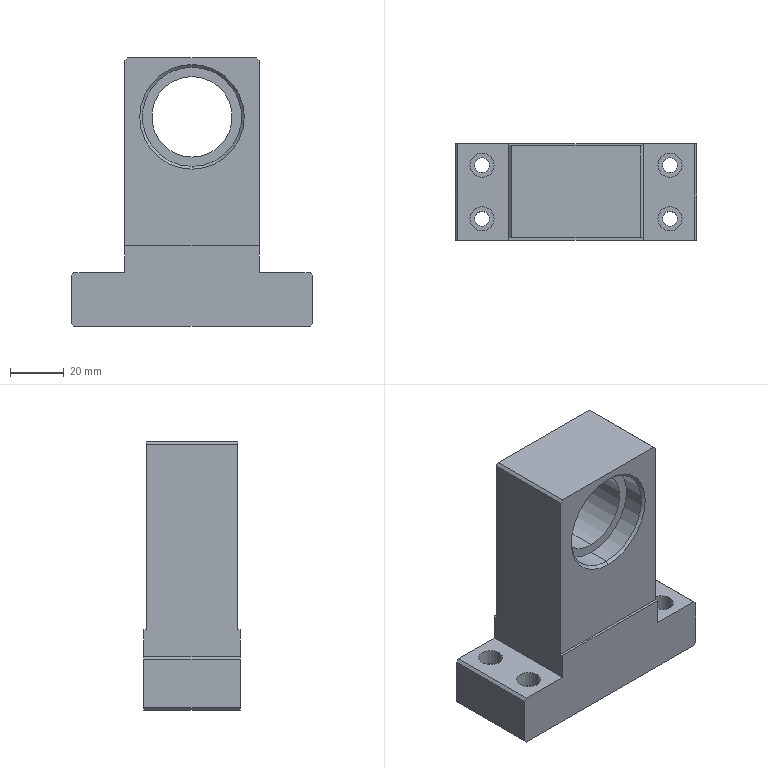Part | NX | features BREP 1 | 1 solid | 68 faces | box 90 x 36 x 100 mm | volume 167256 mm3 | cylinder 30 | plane 26 | cone 12 | commonest cylinder face diameters 4.2 x8 5.5 x8 9 x8 37 x4 30 x2